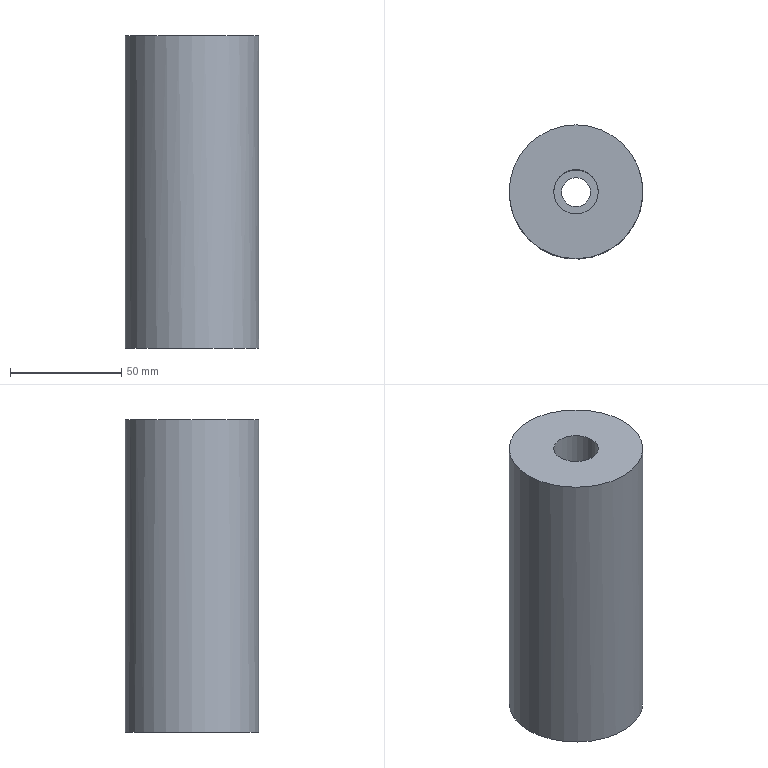Part | NX | features solid 2 | 1 solid | 6 faces | box 60 x 60 x 140 mm | volume 355487 mm3 | cylinder 3 | plane 3 | commonest cylinder face diameters 13 x1 20 x1 60 x1
STEP:
#1=CARTESIAN_POINT('',(-1550.,755.,-80.));
#2=VERTEX_POINT('',#1);
#3=CARTESIAN_POINT('',(-1520.,755.,-80.));
#4=DIRECTION('',(0.,0.,1.));
#5=DIRECTION('',(-1.,0.,0.));
#6=AXIS2_PLACEMENT_3D('',#3,#4,#5);
#7=CIRCLE('',#6,30.);
#8=EDGE_CURVE('',#2,#2,#7,.T.);
#9=ORIENTED_EDGE('',*,*,#8,.T.);
#10=EDGE_LOOP('',(#9));
#11=FACE_BOUND('',#10,.T.);
#12=CARTESIAN_POINT('',(-1490.,755.,60.));
#13=VERTEX_POINT('',#12);
#14=CARTESIAN_POINT('',(-1520.,755.,60.));
#15=DIRECTION('',(0.,0.,1.));
#16=DIRECTION('',(1.,0.,0.));
#17=AXIS2_PLACEMENT_3D('',#14,#15,#16);
#18=CIRCLE('',#17,30.);
#19=EDGE_CURVE('',#13,#13,#18,.T.);
#20=ORIENTED_EDGE('',*,*,#19,.F.);
#21=EDGE_LOOP('',(#20));
#22=FACE_BOUND('',#21,.T.);
#23=CARTESIAN_POINT('',(-1520.,755.,-80.));
#24=DIRECTION('',(0.,0.,1.));
#25=DIRECTION('',(-1.,0.,0.));
#26=AXIS2_PLACEMENT_3D('',#23,#24,#25);
#27=CYLINDRICAL_SURFACE('',#26,30.);
#28=ADVANCED_FACE('',(#11,#22),#27,.T.);
#29=CARTESIAN_POINT('',(-1526.5,755.,-80.));
#30=VERTEX_POINT('',#29);
#31=CARTESIAN_POINT('',(-1520.,755.,-80.));
#32=DIRECTION('',(0.,0.,1.));
#33=DIRECTION('',(-1.,0.,0.));
#34=AXIS2_PLACEMENT_3D('',#31,#32,#33);
#35=CIRCLE('',#34,6.5);
#36=EDGE_CURVE('',#30,#30,#35,.T.);
#37=ORIENTED_EDGE('',*,*,#36,.T.);
#38=EDGE_LOOP('',(#37));
#39=FACE_BOUND('',#38,.T.);
#40=ORIENTED_EDGE('',*,*,#8,.F.);
#41=EDGE_LOOP('',(#40));
#42=FACE_BOUND('',#41,.T.);
#43=CARTESIAN_POINT('',(-1520.,755.,-80.));
#44=DIRECTION('',(0.,0.,1.));
#45=DIRECTION('',(-1.,0.,0.));
#46=AXIS2_PLACEMENT_3D('',#43,#44,#45);
#47=PLANE('',#46);
#48=ADVANCED_FACE('',(#39,#42),#47,.F.);
#49=CARTESIAN_POINT('',(-1510.,755.,60.));
#50=VERTEX_POINT('',#49);
#51=CARTESIAN_POINT('',(-1520.,755.,60.));
#52=DIRECTION('',(0.,0.,1.));
#53=DIRECTION('',(1.,0.,0.));
#54=AXIS2_PLACEMENT_3D('',#51,#52,#53);
#55=CIRCLE('',#54,10.);
#56=EDGE_CURVE('',#50,#50,#55,.F.);
#57=ORIENTED_EDGE('',*,*,#56,.T.);
#58=EDGE_LOOP('',(#57));
#59=FACE_BOUND('',#58,.T.);
#60=ORIENTED_EDGE('',*,*,#19,.T.);
#61=EDGE_LOOP('',(#60));
#62=FACE_BOUND('',#61,.T.);
#63=CARTESIAN_POINT('',(-1520.,755.,60.));
#64=DIRECTION('',(0.,0.,1.));
#65=DIRECTION('',(-1.,0.,0.));
#66=AXIS2_PLACEMENT_3D('',#63,#64,#65);
#67=PLANE('',#66);
#68=ADVANCED_FACE('',(#59,#62),#67,.T.);
#69=CARTESIAN_POINT('',(-1513.5,755.,-60.));
#70=VERTEX_POINT('',#69);
#71=CARTESIAN_POINT('',(-1520.,755.,-60.));
#72=DIRECTION('',(0.,0.,-1.));
#73=DIRECTION('',(1.,0.,0.));
#74=AXIS2_PLACEMENT_3D('',#71,#72,#73);
#75=CIRCLE('',#74,6.5);
#76=EDGE_CURVE('',#70,#70,#75,.T.);
#77=ORIENTED_EDGE('',*,*,#76,.F.);
#78=EDGE_LOOP('',(#77));
#79=FACE_BOUND('',#78,.T.);
#80=ORIENTED_EDGE('',*,*,#36,.F.);
#81=EDGE_LOOP('',(#80));
#82=FACE_BOUND('',#81,.T.);
#83=CARTESIAN_POINT('',(-1520.,755.,-210.));
#84=DIRECTION('',(0.,0.,-1.));
#85=DIRECTION('',(1.,0.,0.));
#86=AXIS2_PLACEMENT_3D('',#83,#84,#85);
#87=CYLINDRICAL_SURFACE('',#86,6.5);
#88=ADVANCED_FACE('',(#79,#82),#87,.F.);
#89=ORIENTED_EDGE('',*,*,#76,.T.);
#90=EDGE_LOOP('',(#89));
#91=FACE_BOUND('',#90,.T.);
#92=CARTESIAN_POINT('',(-1510.,755.,-60.));
#93=VERTEX_POINT('',#92);
#94=CARTESIAN_POINT('',(-1520.,755.,-60.));
#95=DIRECTION('',(0.,0.,-1.));
#96=DIRECTION('',(1.,0.,0.));
#97=AXIS2_PLACEMENT_3D('',#94,#95,#96);
#98=CIRCLE('',#97,10.);
#99=EDGE_CURVE('',#93,#93,#98,.T.);
#100=ORIENTED_EDGE('',*,*,#99,.F.);
#101=EDGE_LOOP('',(#100));
#102=FACE_BOUND('',#101,.T.);
#103=CARTESIAN_POINT('',(-1520.,755.,-60.));
#104=DIRECTION('',(0.,0.,-1.));
#105=DIRECTION('',(1.,0.,0.));
#106=AXIS2_PLACEMENT_3D('',#103,#104,#105);
#107=PLANE('',#106);
#108=ADVANCED_FACE('',(#91,#102),#107,.F.);
#109=ORIENTED_EDGE('',*,*,#99,.T.);
#110=EDGE_LOOP('',(#109));
#111=FACE_BOUND('',#110,.T.);
#112=ORIENTED_EDGE('',*,*,#56,.F.);
#113=EDGE_LOOP('',(#112));
#114=FACE_BOUND('',#113,.T.);
#115=CARTESIAN_POINT('',(-1520.,755.,-10.));
#116=DIRECTION('',(0.,0.,-1.));
#117=DIRECTION('',(1.,0.,0.));
#118=AXIS2_PLACEMENT_3D('',#115,#116,#117);
#119=CYLINDRICAL_SURFACE('',#118,10.);
#120=ADVANCED_FACE('',(#111,#114),#119,.F.);
#121=CLOSED_SHELL('',(#28,#48,#68,#88,#108,#120));
#122=MANIFOLD_SOLID_BREP('',#121);
#123=(LENGTH_UNIT()NAMED_UNIT(*)SI_UNIT(.MILLI.,.METRE.));
#124=UNCERTAINTY_MEASURE_WITH_UNIT(LENGTH_MEASURE(0.00001),#123,'','');
#125=(NAMED_UNIT(*)PLANE_ANGLE_UNIT()SI_UNIT($,.RADIAN.));
#126=(NAMED_UNIT(*)SI_UNIT($,.STERADIAN.)SOLID_ANGLE_UNIT());
#127=(GEOMETRIC_REPRESENTATION_CONTEXT(3)GLOBAL_UNCERTAINTY_ASSIGNED_CONTEXT((#124))GLOBAL_UNIT_ASSIGNED_CONTEXT((#123,#125,#126))REPRESENTATION_CONTEXT('',''));
#128=ADVANCED_BREP_SHAPE_REPRESENTATION('',(#122),#127);